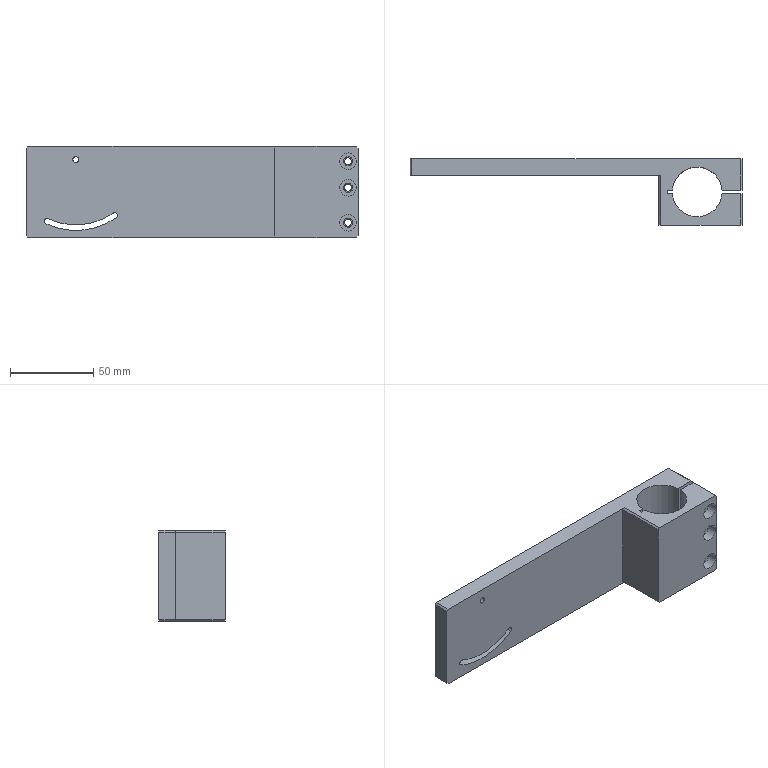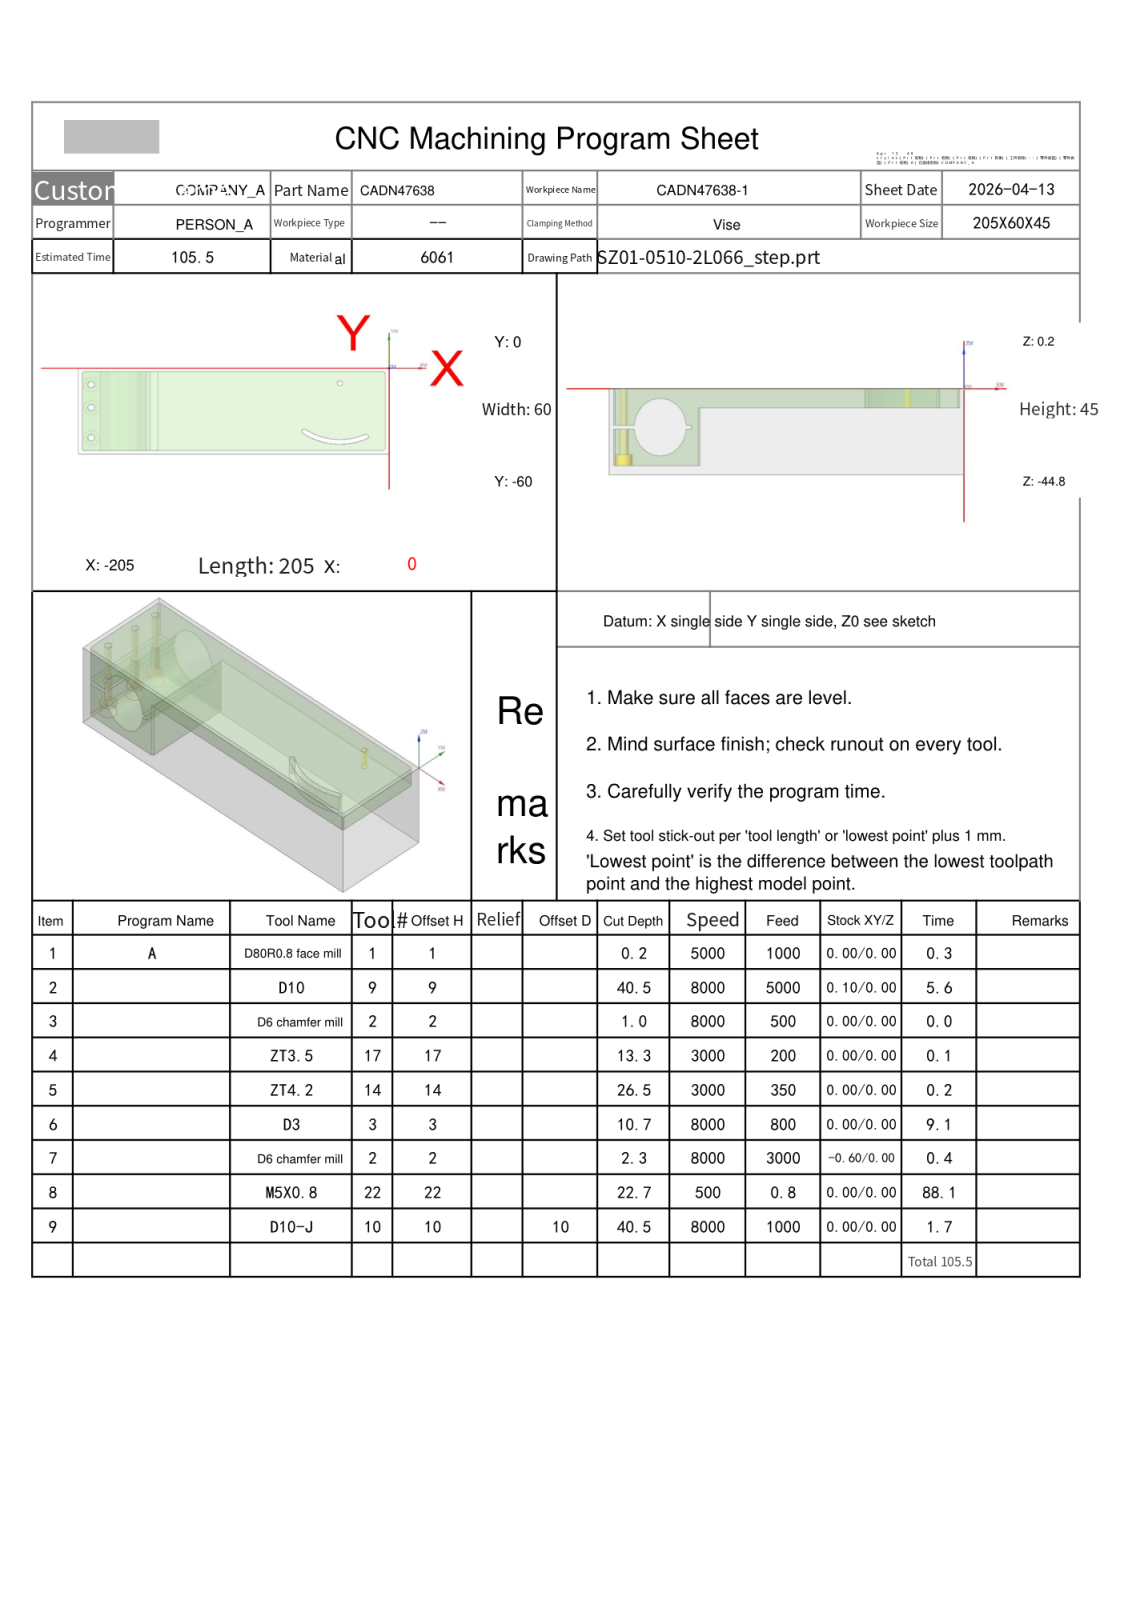NC program | NX | posted by the shop | part box 200 x 40 x 55 mm
Lines 1 to 1033 of 2500:
%
O0001
(Machine time: 191.78 MIN)
(===Total Tool:8===)
(T1=D80R0.8 face mill D=80. R=0.8 D-H01 Z=0.    )
(T9=D10     D=10.  R=0.   D-  H09 Z=-40.3 )
(T2=D6 chamfer mill D=6. R=0. D-H02 Z=-2.05 )
(T17=ZT3.5  D=3.5  DR_a=118 D-  H17 Z=-13.05)
(T14=ZT4.2  D=4.2  DR_a=118 D-  H14 Z=-26.26)
(T3=D3      D=3.   R=0.   D3  H03 Z=-10.5 )
(T22=M5X0.8 D=4.2  DR_a=180 D-  H22 Z=-22.5 )
(T10=D10-J  D=10.  R=0.   D10 H10 Z=-40.3 )
G80 G90 G17 G49 G40
G91 G28 Z0
M01
N1 T01 M06
(D80R0.8 face mill D=80. R=0.8 H=01 ce=0.00 di=0.00)
(MAX_Z=20. MIN_Z=0. Time=0.31M)
G00 G90 G54 X-247.5 Y-30. M03 S5000
G43 H01 Z20.
M08
Z2.
G01 Z0.0 F1000.
X-242.5
X37.5
X42.5
Z2.
G00 Z20.
G91 G28 Z0.0
M05
M09
G91 G28 Z0.0
M01
N2 T09 M06
(D10  D=10. R=0. H=09 ce=0.10 di=0.00)
(MAX_Z=20. MIN_Z=-40.3 Time=5.63M)
G00 G90 G54 X-102.622 Y-62.6 M03 S8000
G43 H09 Z20.
M08
Z.5
G01 X-201.5 Z.353 F5000.
G02 X-201.744 Y-62.594 Z.353 I0.0 J5.1
X-205.106 Y-61.106 Z.347 I.244 J5.094
G01 X-206.106 Y-60.106 Z.345
G02 X-207.6 Y-56.5 Z.339 I3.606 J3.606
G01 Y-3.5 Z.261
G02 X-206.106 Y.106 Z.255 I5.1 J0.0
G01 X-205.106 Y1.106 Z.253
G02 X-201.744 Y2.594 Z.247 I3.606 J-3.606
X-201.5 Y2.6 Z.247 I.244 J-5.094
G01 X-3.5 Z-.047
G02 X.106 Y1.106 Z-.053 I0.0 J-5.1
G01 X1.106 Y.106 Z-.055
G02 X2.6 Y-3.5 Z-.061 I-3.606 J-3.606
G01 Y-56.5 Z-.139
G02 X1.106 Y-60.106 Z-.145 I-5.1 J0.0
G01 X.106 Y-61.106 Z-.147
G02 X-3.5 Y-62.6 Z-.153 I-3.606 J3.606
G01 X-201.5 Z-.447
G02 X-201.744 Y-62.594 Z-.447 I0.0 J5.1
X-205.106 Y-61.106 Z-.453 I.244 J5.094
G01 X-206.106 Y-60.106 Z-.455
G02 X-207.6 Y-56.5 Z-.461 I3.606 J3.606
G01 Y-3.5 Z-.539
G02 X-206.106 Y.106 Z-.545 I5.1 J0.0
G01 X-205.106 Y1.106 Z-.547
G02 X-201.744 Y2.594 Z-.553 I3.606 J-3.606
X-201.5 Y2.6 Z-.553 I.244 J-5.094
G01 X-3.5 Z-.847
G02 X.106 Y1.106 Z-.853 I0.0 J-5.1
G01 X1.106 Y.106 Z-.855
G02 X2.6 Y-3.5 Z-.861 I-3.606 J-3.606
G01 Y-56.5 Z-.939
G02 X1.106 Y-60.106 Z-.945 I-5.1 J0.0
G01 X.106 Y-61.106 Z-.947
G02 X-3.5 Y-62.6 Z-.953 I-3.606 J3.606
G01 X-201.5 Z-1.247
G02 X-201.744 Y-62.594 Z-1.247 I0.0 J5.1
X-205.106 Y-61.106 Z-1.253 I.244 J5.094
G01 X-206.106 Y-60.106 Z-1.255
G02 X-207.6 Y-56.5 Z-1.261 I3.606 J3.606
G01 Y-3.5 Z-1.339
G02 X-206.106 Y.106 Z-1.345 I5.1 J0.0
G01 X-205.106 Y1.106 Z-1.347
G02 X-201.744 Y2.594 Z-1.353 I3.606 J-3.606
X-201.5 Y2.6 Z-1.353 I.244 J-5.094
G01 X-3.5 Z-1.647
G02 X.106 Y1.106 Z-1.653 I0.0 J-5.1
G01 X1.106 Y.106 Z-1.655
G02 X2.6 Y-3.5 Z-1.661 I-3.606 J-3.606
G01 Y-56.5 Z-1.739
G02 X1.106 Y-60.106 Z-1.745 I-5.1 J0.0
G01 X.106 Y-61.106 Z-1.747
G02 X-3.5 Y-62.6 Z-1.753 I-3.606 J3.606
G01 X-201.5 Z-2.047
G02 X-201.744 Y-62.594 Z-2.047 I0.0 J5.1
X-205.106 Y-61.106 Z-2.053 I.244 J5.094
G01 X-206.106 Y-60.106 Z-2.055
G02 X-207.6 Y-56.5 Z-2.061 I3.606 J3.606
G01 Y-3.5 Z-2.139
G02 X-206.106 Y.106 Z-2.145 I5.1 J0.0
G01 X-205.106 Y1.106 Z-2.147
G02 X-201.744 Y2.594 Z-2.153 I3.606 J-3.606
X-201.5 Y2.6 Z-2.153 I.244 J-5.094
G01 X-3.5 Z-2.447
G02 X.106 Y1.106 Z-2.453 I0.0 J-5.1
G01 X1.106 Y.106 Z-2.455
G02 X2.6 Y-3.5 Z-2.461 I-3.606 J-3.606
G01 Y-56.5 Z-2.539
G02 X1.106 Y-60.106 Z-2.545 I-5.1 J0.0
G01 X.106 Y-61.106 Z-2.547
G02 X-3.5 Y-62.6 Z-2.553 I-3.606 J3.606
G01 X-201.5 Z-2.847
G02 X-201.744 Y-62.594 Z-2.847 I0.0 J5.1
X-205.106 Y-61.106 Z-2.853 I.244 J5.094
G01 X-206.106 Y-60.106 Z-2.855
G02 X-207.6 Y-56.5 Z-2.861 I3.606 J3.606
G01 Y-3.5 Z-2.939
G02 X-206.106 Y.106 Z-2.945 I5.1 J0.0
G01 X-205.106 Y1.106 Z-2.947
G02 X-201.744 Y2.594 Z-2.953 I3.606 J-3.606
X-201.5 Y2.6 Z-2.953 I.244 J-5.094
G01 X-3.5 Z-3.247
G02 X.106 Y1.106 Z-3.253 I0.0 J-5.1
G01 X1.106 Y.106 Z-3.255
G02 X2.6 Y-3.5 Z-3.261 I-3.606 J-3.606
G01 Y-56.5 Z-3.339
G02 X1.106 Y-60.106 Z-3.345 I-5.1 J0.0
G01 X.106 Y-61.106 Z-3.347
G02 X-3.5 Y-62.6 Z-3.353 I-3.606 J3.606
G01 X-201.5 Z-3.647
G02 X-201.744 Y-62.594 Z-3.647 I0.0 J5.1
X-205.106 Y-61.106 Z-3.653 I.244 J5.094
G01 X-206.106 Y-60.106 Z-3.655
G02 X-207.6 Y-56.5 Z-3.661 I3.606 J3.606
G01 Y-3.5 Z-3.739
G02 X-206.106 Y.106 Z-3.745 I5.1 J0.0
G01 X-205.106 Y1.106 Z-3.747
G02 X-201.744 Y2.594 Z-3.753 I3.606 J-3.606
X-201.5 Y2.6 Z-3.753 I.244 J-5.094
G01 X-3.5 Z-4.047
G02 X.106 Y1.106 Z-4.053 I0.0 J-5.1
G01 X1.106 Y.106 Z-4.055
G02 X2.6 Y-3.5 Z-4.061 I-3.606 J-3.606
G01 Y-56.5 Z-4.139
G02 X1.106 Y-60.106 Z-4.145 I-5.1 J0.0
G01 X.106 Y-61.106 Z-4.147
G02 X-3.5 Y-62.6 Z-4.153 I-3.606 J3.606
G01 X-201.5 Z-4.447
G02 X-201.744 Y-62.594 Z-4.447 I0.0 J5.1
X-205.106 Y-61.106 Z-4.453 I.244 J5.094
G01 X-206.106 Y-60.106 Z-4.455
G02 X-207.6 Y-56.5 Z-4.461 I3.606 J3.606
G01 Y-3.5 Z-4.539
G02 X-206.106 Y.106 Z-4.545 I5.1 J0.0
G01 X-205.106 Y1.106 Z-4.547
G02 X-201.744 Y2.594 Z-4.553 I3.606 J-3.606
X-201.5 Y2.6 Z-4.553 I.244 J-5.094
G01 X-3.5 Z-4.847
G02 X.106 Y1.106 Z-4.853 I0.0 J-5.1
G01 X1.106 Y.106 Z-4.855
G02 X2.6 Y-3.5 Z-4.861 I-3.606 J-3.606
G01 Y-56.5 Z-4.939
G02 X1.106 Y-60.106 Z-4.945 I-5.1 J0.0
G01 X.106 Y-61.106 Z-4.947
G02 X-3.5 Y-62.6 Z-4.953 I-3.606 J3.606
G01 X-201.5 Z-5.247
G02 X-201.744 Y-62.594 Z-5.247 I0.0 J5.1
X-205.106 Y-61.106 Z-5.253 I.244 J5.094
G01 X-206.106 Y-60.106 Z-5.255
G02 X-207.6 Y-56.5 Z-5.261 I3.606 J3.606
G01 Y-3.5 Z-5.339
G02 X-206.106 Y.106 Z-5.345 I5.1 J0.0
G01 X-205.106 Y1.106 Z-5.347
G02 X-201.744 Y2.594 Z-5.353 I3.606 J-3.606
X-201.5 Y2.6 Z-5.353 I.244 J-5.094
G01 X-3.5 Z-5.647
G02 X.106 Y1.106 Z-5.653 I0.0 J-5.1
G01 X1.106 Y.106 Z-5.655
G02 X2.6 Y-3.5 Z-5.661 I-3.606 J-3.606
G01 Y-56.5 Z-5.739
G02 X1.106 Y-60.106 Z-5.745 I-5.1 J0.0
G01 X.106 Y-61.106 Z-5.747
G02 X-3.5 Y-62.6 Z-5.753 I-3.606 J3.606
G01 X-201.5 Z-6.047
G02 X-201.744 Y-62.594 Z-6.047 I0.0 J5.1
X-205.106 Y-61.106 Z-6.053 I.244 J5.094
G01 X-206.106 Y-60.106 Z-6.055
G02 X-207.6 Y-56.5 Z-6.061 I3.606 J3.606
G01 Y-3.5 Z-6.139
G02 X-206.106 Y.106 Z-6.145 I5.1 J0.0
G01 X-205.106 Y1.106 Z-6.147
G02 X-201.744 Y2.594 Z-6.153 I3.606 J-3.606
X-201.5 Y2.6 Z-6.153 I.244 J-5.094
G01 X-3.5 Z-6.447
G02 X.106 Y1.106 Z-6.453 I0.0 J-5.1
G01 X1.106 Y.106 Z-6.455
G02 X2.6 Y-3.5 Z-6.461 I-3.606 J-3.606
G01 Y-56.5 Z-6.539
G02 X1.106 Y-60.106 Z-6.545 I-5.1 J0.0
G01 X.106 Y-61.106 Z-6.547
G02 X-3.5 Y-62.6 Z-6.553 I-3.606 J3.606
G01 X-201.5 Z-6.847
G02 X-201.744 Y-62.594 Z-6.847 I0.0 J5.1
X-205.106 Y-61.106 Z-6.853 I.244 J5.094
G01 X-206.106 Y-60.106 Z-6.855
G02 X-207.6 Y-56.5 Z-6.861 I3.606 J3.606
G01 Y-3.5 Z-6.939
G02 X-206.106 Y.106 Z-6.945 I5.1 J0.0
G01 X-205.106 Y1.106 Z-6.947
G02 X-201.744 Y2.594 Z-6.953 I3.606 J-3.606
X-201.5 Y2.6 Z-6.953 I.244 J-5.094
G01 X-3.5 Z-7.247
G02 X.106 Y1.106 Z-7.253 I0.0 J-5.1
G01 X1.106 Y.106 Z-7.255
G02 X2.6 Y-3.5 Z-7.261 I-3.606 J-3.606
G01 Y-56.5 Z-7.339
G02 X1.106 Y-60.106 Z-7.345 I-5.1 J0.0
G01 X.106 Y-61.106 Z-7.347
G02 X-3.5 Y-62.6 Z-7.353 I-3.606 J3.606
G01 X-201.5 Z-7.647
G02 X-201.744 Y-62.594 Z-7.647 I0.0 J5.1
X-205.106 Y-61.106 Z-7.653 I.244 J5.094
G01 X-206.106 Y-60.106 Z-7.655
G02 X-207.6 Y-56.5 Z-7.661 I3.606 J3.606
G01 Y-3.5 Z-7.739
G02 X-206.106 Y.106 Z-7.745 I5.1 J0.0
G01 X-205.106 Y1.106 Z-7.747
G02 X-201.744 Y2.594 Z-7.753 I3.606 J-3.606
X-201.5 Y2.6 Z-7.753 I.244 J-5.094
G01 X-3.5 Z-8.047
G02 X.106 Y1.106 Z-8.053 I0.0 J-5.1
G01 X1.106 Y.106 Z-8.055
G02 X2.6 Y-3.5 Z-8.061 I-3.606 J-3.606
G01 Y-56.5 Z-8.139
G02 X1.106 Y-60.106 Z-8.145 I-5.1 J0.0
G01 X.106 Y-61.106 Z-8.147
G02 X-3.5 Y-62.6 Z-8.153 I-3.606 J3.606
G01 X-201.5 Z-8.447
G02 X-201.744 Y-62.594 Z-8.447 I0.0 J5.1
X-205.106 Y-61.106 Z-8.453 I.244 J5.094
G01 X-206.106 Y-60.106 Z-8.455
G02 X-207.6 Y-56.5 Z-8.461 I3.606 J3.606
G01 Y-3.5 Z-8.539
G02 X-206.106 Y.106 Z-8.545 I5.1 J0.0
G01 X-205.106 Y1.106 Z-8.547
G02 X-201.744 Y2.594 Z-8.553 I3.606 J-3.606
X-201.5 Y2.6 Z-8.553 I.244 J-5.094
G01 X-3.5 Z-8.847
G02 X.106 Y1.106 Z-8.853 I0.0 J-5.1
G01 X1.106 Y.106 Z-8.855
G02 X2.6 Y-3.5 Z-8.861 I-3.606 J-3.606
G01 Y-56.5 Z-8.939
G02 X1.106 Y-60.106 Z-8.945 I-5.1 J0.0
G01 X.106 Y-61.106 Z-8.947
G02 X-3.5 Y-62.6 Z-8.953 I-3.606 J3.606
G01 X-201.5 Z-9.247
G02 X-201.744 Y-62.594 Z-9.247 I0.0 J5.1
X-205.106 Y-61.106 Z-9.253 I.244 J5.094
G01 X-206.106 Y-60.106 Z-9.255
G02 X-207.6 Y-56.5 Z-9.261 I3.606 J3.606
G01 Y-3.5 Z-9.339
G02 X-206.106 Y.106 Z-9.345 I5.1 J0.0
G01 X-205.106 Y1.106 Z-9.347
G02 X-201.744 Y2.594 Z-9.353 I3.606 J-3.606
X-201.5 Y2.6 Z-9.353 I.244 J-5.094
G01 X-3.5 Z-9.647
G02 X.106 Y1.106 Z-9.653 I0.0 J-5.1
G01 X1.106 Y.106 Z-9.655
G02 X2.6 Y-3.5 Z-9.661 I-3.606 J-3.606
G01 Y-56.5 Z-9.739
G02 X1.106 Y-60.106 Z-9.745 I-5.1 J0.0
G01 X.106 Y-61.106 Z-9.747
G02 X-3.5 Y-62.6 Z-9.753 I-3.606 J3.606
G01 X-201.5 Z-10.047
G02 X-201.744 Y-62.594 Z-10.047 I0.0 J5.1
X-205.106 Y-61.106 Z-10.053 I.244 J5.094
G01 X-206.106 Y-60.106 Z-10.055
G02 X-207.6 Y-56.5 Z-10.061 I3.606 J3.606
G01 Y-3.5 Z-10.139
G02 X-206.106 Y.106 Z-10.145 I5.1 J0.0
G01 X-205.106 Y1.106 Z-10.147
G02 X-201.744 Y2.594 Z-10.153 I3.606 J-3.606
X-201.5 Y2.6 Z-10.153 I.244 J-5.094
G01 X-3.5 Z-10.447
G02 X.106 Y1.106 Z-10.453 I0.0 J-5.1
G01 X1.106 Y.106 Z-10.455
G02 X2.6 Y-3.5 Z-10.461 I-3.606 J-3.606
G01 Y-56.5 Z-10.539
G02 X1.106 Y-60.106 Z-10.545 I-5.1 J0.0
G01 X.106 Y-61.106 Z-10.547
G02 X-3.5 Y-62.6 Z-10.553 I-3.606 J3.606
G01 X-201.5 Z-10.847
G02 X-201.744 Y-62.594 Z-10.847 I0.0 J5.1
X-205.106 Y-61.106 Z-10.853 I.244 J5.094
G01 X-206.106 Y-60.106 Z-10.855
G02 X-207.6 Y-56.5 Z-10.861 I3.606 J3.606
G01 Y-3.5 Z-10.939
G02 X-206.106 Y.106 Z-10.945 I5.1 J0.0
G01 X-205.106 Y1.106 Z-10.947
G02 X-201.744 Y2.594 Z-10.953 I3.606 J-3.606
X-201.5 Y2.6 Z-10.953 I.244 J-5.094
G01 X-3.5 Z-11.247
G02 X.106 Y1.106 Z-11.253 I0.0 J-5.1
G01 X1.106 Y.106 Z-11.255
G02 X2.6 Y-3.5 Z-11.261 I-3.606 J-3.606
G01 Y-56.5 Z-11.339
G02 X1.106 Y-60.106 Z-11.345 I-5.1 J0.0
G01 X.106 Y-61.106 Z-11.347
G02 X-3.5 Y-62.6 Z-11.353 I-3.606 J3.606
G01 X-201.5 Z-11.647
G02 X-201.744 Y-62.594 Z-11.647 I0.0 J5.1
X-205.106 Y-61.106 Z-11.653 I.244 J5.094
G01 X-206.106 Y-60.106 Z-11.655
G02 X-207.6 Y-56.5 Z-11.661 I3.606 J3.606
G01 Y-3.5 Z-11.739
G02 X-206.106 Y.106 Z-11.745 I5.1 J0.0
G01 X-205.106 Y1.106 Z-11.747
G02 X-201.744 Y2.594 Z-11.753 I3.606 J-3.606
X-201.5 Y2.6 Z-11.753 I.244 J-5.094
G01 X-3.5 Z-12.047
G02 X.106 Y1.106 Z-12.053 I0.0 J-5.1
G01 X1.106 Y.106 Z-12.055
G02 X2.6 Y-3.5 Z-12.061 I-3.606 J-3.606
G01 Y-56.5 Z-12.139
G02 X1.106 Y-60.106 Z-12.145 I-5.1 J0.0
G01 X.106 Y-61.106 Z-12.147
G02 X-3.5 Y-62.6 Z-12.153 I-3.606 J3.606
G01 X-201.5 Z-12.447
G02 X-201.744 Y-62.594 Z-12.447 I0.0 J5.1
X-205.106 Y-61.106 Z-12.453 I.244 J5.094
G01 X-206.106 Y-60.106 Z-12.455
G02 X-207.6 Y-56.5 Z-12.461 I3.606 J3.606
G01 Y-3.5 Z-12.539
G02 X-206.106 Y.106 Z-12.545 I5.1 J0.0
G01 X-205.106 Y1.106 Z-12.547
G02 X-201.744 Y2.594 Z-12.553 I3.606 J-3.606
X-201.5 Y2.6 Z-12.553 I.244 J-5.094
G01 X-3.5 Z-12.847
G02 X.106 Y1.106 Z-12.853 I0.0 J-5.1
G01 X1.106 Y.106 Z-12.855
G02 X2.6 Y-3.5 Z-12.861 I-3.606 J-3.606
G01 Y-56.5 Z-12.939
G02 X1.106 Y-60.106 Z-12.945 I-5.1 J0.0
G01 X.106 Y-61.106 Z-12.947
G02 X-3.5 Y-62.6 Z-12.953 I-3.606 J3.606
G01 X-201.5 Z-13.247
G02 X-201.744 Y-62.594 Z-13.247 I0.0 J5.1
X-205.106 Y-61.106 Z-13.253 I.244 J5.094
G01 X-206.106 Y-60.106 Z-13.255
G02 X-207.6 Y-56.5 Z-13.261 I3.606 J3.606
G01 Y-3.5 Z-13.339
G02 X-206.106 Y.106 Z-13.345 I5.1 J0.0
G01 X-205.106 Y1.106 Z-13.347
G02 X-201.744 Y2.594 Z-13.353 I3.606 J-3.606
X-201.5 Y2.6 Z-13.353 I.244 J-5.094
G01 X-3.5 Z-13.647
G02 X.106 Y1.106 Z-13.653 I0.0 J-5.1
G01 X1.106 Y.106 Z-13.655
G02 X2.6 Y-3.5 Z-13.661 I-3.606 J-3.606
G01 Y-56.5 Z-13.739
G02 X1.106 Y-60.106 Z-13.745 I-5.1 J0.0
G01 X.106 Y-61.106 Z-13.747
G02 X-3.5 Y-62.6 Z-13.753 I-3.606 J3.606
G01 X-201.5 Z-14.047
G02 X-201.744 Y-62.594 Z-14.047 I0.0 J5.1
X-205.106 Y-61.106 Z-14.053 I.244 J5.094
G01 X-206.106 Y-60.106 Z-14.055
G02 X-207.6 Y-56.5 Z-14.061 I3.606 J3.606
G01 Y-3.5 Z-14.139
G02 X-206.106 Y.106 Z-14.145 I5.1 J0.0
G01 X-205.106 Y1.106 Z-14.147
G02 X-201.744 Y2.594 Z-14.153 I3.606 J-3.606
X-201.5 Y2.6 Z-14.153 I.244 J-5.094
G01 X-3.5 Z-14.447
G02 X.106 Y1.106 Z-14.453 I0.0 J-5.1
G01 X1.106 Y.106 Z-14.455
G02 X2.6 Y-3.5 Z-14.461 I-3.606 J-3.606
G01 Y-56.5 Z-14.539
G02 X1.106 Y-60.106 Z-14.545 I-5.1 J0.0
G01 X.106 Y-61.106 Z-14.547
G02 X-3.5 Y-62.6 Z-14.553 I-3.606 J3.606
G01 X-201.5 Z-14.847
G02 X-201.744 Y-62.594 Z-14.847 I0.0 J5.1
X-205.106 Y-61.106 Z-14.853 I.244 J5.094
G01 X-206.106 Y-60.106 Z-14.855
G02 X-207.6 Y-56.5 Z-14.861 I3.606 J3.606
G01 Y-3.5 Z-14.939
G02 X-206.106 Y.106 Z-14.945 I5.1 J0.0
G01 X-205.106 Y1.106 Z-14.947
G02 X-201.744 Y2.594 Z-14.953 I3.606 J-3.606
X-201.5 Y2.6 Z-14.953 I.244 J-5.094
G01 X-3.5 Z-15.247
G02 X.106 Y1.106 Z-15.253 I0.0 J-5.1
G01 X1.106 Y.106 Z-15.255
G02 X2.6 Y-3.5 Z-15.261 I-3.606 J-3.606
G01 Y-56.5 Z-15.339
G02 X1.106 Y-60.106 Z-15.345 I-5.1 J0.0
G01 X.106 Y-61.106 Z-15.347
G02 X-3.5 Y-62.6 Z-15.353 I-3.606 J3.606
G01 X-201.5 Z-15.647
G02 X-201.744 Y-62.594 Z-15.647 I0.0 J5.1
X-205.106 Y-61.106 Z-15.653 I.244 J5.094
G01 X-206.106 Y-60.106 Z-15.655
G02 X-207.6 Y-56.5 Z-15.661 I3.606 J3.606
G01 Y-3.5 Z-15.739
G02 X-206.106 Y.106 Z-15.745 I5.1 J0.0
G01 X-205.106 Y1.106 Z-15.747
G02 X-201.744 Y2.594 Z-15.753 I3.606 J-3.606
X-201.5 Y2.6 Z-15.753 I.244 J-5.094
G01 X-3.5 Z-16.047
G02 X.106 Y1.106 Z-16.053 I0.0 J-5.1
G01 X1.106 Y.106 Z-16.055
G02 X2.6 Y-3.5 Z-16.061 I-3.606 J-3.606
G01 Y-56.5 Z-16.139
G02 X1.106 Y-60.106 Z-16.145 I-5.1 J0.0
G01 X.106 Y-61.106 Z-16.147
G02 X-3.5 Y-62.6 Z-16.153 I-3.606 J3.606
G01 X-201.5 Z-16.447
G02 X-201.744 Y-62.594 Z-16.447 I0.0 J5.1
X-205.106 Y-61.106 Z-16.453 I.244 J5.094
G01 X-206.106 Y-60.106 Z-16.455
G02 X-207.6 Y-56.5 Z-16.461 I3.606 J3.606
G01 Y-3.5 Z-16.539
G02 X-206.106 Y.106 Z-16.545 I5.1 J0.0
G01 X-205.106 Y1.106 Z-16.547
G02 X-201.744 Y2.594 Z-16.553 I3.606 J-3.606
X-201.5 Y2.6 Z-16.553 I.244 J-5.094
G01 X-3.5 Z-16.847
G02 X.106 Y1.106 Z-16.853 I0.0 J-5.1
G01 X1.106 Y.106 Z-16.855
G02 X2.6 Y-3.5 Z-16.861 I-3.606 J-3.606
G01 Y-56.5 Z-16.939
G02 X1.106 Y-60.106 Z-16.945 I-5.1 J0.0
G01 X.106 Y-61.106 Z-16.947
G02 X-3.5 Y-62.6 Z-16.953 I-3.606 J3.606
G01 X-201.5 Z-17.247
G02 X-201.744 Y-62.594 Z-17.247 I0.0 J5.1
X-205.106 Y-61.106 Z-17.253 I.244 J5.094
G01 X-206.106 Y-60.106 Z-17.255
G02 X-207.6 Y-56.5 Z-17.261 I3.606 J3.606
G01 Y-3.5 Z-17.339
G02 X-206.106 Y.106 Z-17.345 I5.1 J0.0
G01 X-205.106 Y1.106 Z-17.347
G02 X-201.744 Y2.594 Z-17.353 I3.606 J-3.606
X-201.5 Y2.6 Z-17.353 I.244 J-5.094
G01 X-3.5 Z-17.647
G02 X.106 Y1.106 Z-17.653 I0.0 J-5.1
G01 X1.106 Y.106 Z-17.655
G02 X2.6 Y-3.5 Z-17.661 I-3.606 J-3.606
G01 Y-56.5 Z-17.739
G02 X1.106 Y-60.106 Z-17.745 I-5.1 J0.0
G01 X.106 Y-61.106 Z-17.747
G02 X-3.5 Y-62.6 Z-17.753 I-3.606 J3.606
G01 X-201.5 Z-18.047
G02 X-201.744 Y-62.594 Z-18.047 I0.0 J5.1
X-205.106 Y-61.106 Z-18.053 I.244 J5.094
G01 X-206.106 Y-60.106 Z-18.055
G02 X-207.6 Y-56.5 Z-18.061 I3.606 J3.606
G01 Y-3.5 Z-18.139
G02 X-206.106 Y.106 Z-18.145 I5.1 J0.0
G01 X-205.106 Y1.106 Z-18.147
G02 X-201.744 Y2.594 Z-18.153 I3.606 J-3.606
X-201.5 Y2.6 Z-18.153 I.244 J-5.094
G01 X-3.5 Z-18.447
G02 X.106 Y1.106 Z-18.453 I0.0 J-5.1
G01 X1.106 Y.106 Z-18.455
G02 X2.6 Y-3.5 Z-18.461 I-3.606 J-3.606
G01 Y-56.5 Z-18.539
G02 X1.106 Y-60.106 Z-18.545 I-5.1 J0.0
G01 X.106 Y-61.106 Z-18.547
G02 X-3.5 Y-62.6 Z-18.553 I-3.606 J3.606
G01 X-201.5 Z-18.847
G02 X-201.744 Y-62.594 Z-18.847 I0.0 J5.1
X-205.106 Y-61.106 Z-18.853 I.244 J5.094
G01 X-206.106 Y-60.106 Z-18.855
G02 X-207.6 Y-56.5 Z-18.861 I3.606 J3.606
G01 Y-3.5 Z-18.939
G02 X-206.106 Y.106 Z-18.945 I5.1 J0.0
G01 X-205.106 Y1.106 Z-18.947
G02 X-201.744 Y2.594 Z-18.953 I3.606 J-3.606
X-201.5 Y2.6 Z-18.953 I.244 J-5.094
G01 X-3.5 Z-19.247
G02 X.106 Y1.106 Z-19.253 I0.0 J-5.1
G01 X1.106 Y.106 Z-19.255
G02 X2.6 Y-3.5 Z-19.261 I-3.606 J-3.606
G01 Y-56.5 Z-19.339
G02 X1.106 Y-60.106 Z-19.345 I-5.1 J0.0
G01 X.106 Y-61.106 Z-19.347
G02 X-3.5 Y-62.6 Z-19.353 I-3.606 J3.606
G01 X-201.5 Z-19.647
G02 X-201.744 Y-62.594 Z-19.647 I0.0 J5.1
X-205.106 Y-61.106 Z-19.653 I.244 J5.094
G01 X-206.106 Y-60.106 Z-19.655
G02 X-207.6 Y-56.5 Z-19.661 I3.606 J3.606
G01 Y-3.5 Z-19.739
G02 X-206.106 Y.106 Z-19.745 I5.1 J0.0
G01 X-205.106 Y1.106 Z-19.747
G02 X-201.744 Y2.594 Z-19.753 I3.606 J-3.606
X-201.5 Y2.6 Z-19.753 I.244 J-5.094
G01 X-3.5 Z-20.047
G02 X.106 Y1.106 Z-20.053 I0.0 J-5.1
G01 X1.106 Y.106 Z-20.055
G02 X2.6 Y-3.5 Z-20.061 I-3.606 J-3.606
G01 Y-56.5 Z-20.139
G02 X1.106 Y-60.106 Z-20.145 I-5.1 J0.0
G01 X.106 Y-61.106 Z-20.147
G02 X-3.5 Y-62.6 Z-20.153 I-3.606 J3.606
G01 X-201.5 Z-20.447
G02 X-201.744 Y-62.594 Z-20.447 I0.0 J5.1
X-205.106 Y-61.106 Z-20.453 I.244 J5.094
G01 X-206.106 Y-60.106 Z-20.455
G02 X-207.6 Y-56.5 Z-20.461 I3.606 J3.606
G01 Y-3.5 Z-20.539
G02 X-206.106 Y.106 Z-20.545 I5.1 J0.0
G01 X-205.106 Y1.106 Z-20.547
G02 X-201.744 Y2.594 Z-20.553 I3.606 J-3.606
X-201.5 Y2.6 Z-20.553 I.244 J-5.094
G01 X-3.5 Z-20.847
G02 X.106 Y1.106 Z-20.853 I0.0 J-5.1
G01 X1.106 Y.106 Z-20.855
G02 X2.6 Y-3.5 Z-20.861 I-3.606 J-3.606
G01 Y-56.5 Z-20.939
G02 X1.106 Y-60.106 Z-20.945 I-5.1 J0.0
G01 X.106 Y-61.106 Z-20.947
G02 X-3.5 Y-62.6 Z-20.953 I-3.606 J3.606
G01 X-201.5 Z-21.247
G02 X-201.744 Y-62.594 Z-21.247 I0.0 J5.1
X-205.106 Y-61.106 Z-21.253 I.244 J5.094
G01 X-206.106 Y-60.106 Z-21.255
G02 X-207.6 Y-56.5 Z-21.261 I3.606 J3.606
G01 Y-3.5 Z-21.339
G02 X-206.106 Y.106 Z-21.345 I5.1 J0.0
G01 X-205.106 Y1.106 Z-21.347
G02 X-201.744 Y2.594 Z-21.353 I3.606 J-3.606
X-201.5 Y2.6 Z-21.353 I.244 J-5.094
G01 X-3.5 Z-21.647
G02 X.106 Y1.106 Z-21.653 I0.0 J-5.1
G01 X1.106 Y.106 Z-21.655
G02 X2.6 Y-3.5 Z-21.661 I-3.606 J-3.606
G01 Y-56.5 Z-21.739
G02 X1.106 Y-60.106 Z-21.745 I-5.1 J0.0
G01 X.106 Y-61.106 Z-21.747
G02 X-3.5 Y-62.6 Z-21.753 I-3.606 J3.606
G01 X-201.5 Z-22.047
G02 X-201.744 Y-62.594 Z-22.047 I0.0 J5.1
X-205.106 Y-61.106 Z-22.053 I.244 J5.094
G01 X-206.106 Y-60.106 Z-22.055
G02 X-207.6 Y-56.5 Z-22.061 I3.606 J3.606
G01 Y-3.5 Z-22.139
G02 X-206.106 Y.106 Z-22.145 I5.1 J0.0
G01 X-205.106 Y1.106 Z-22.147
G02 X-201.744 Y2.594 Z-22.153 I3.606 J-3.606
X-201.5 Y2.6 Z-22.153 I.244 J-5.094
G01 X-3.5 Z-22.447
G02 X.106 Y1.106 Z-22.453 I0.0 J-5.1
G01 X1.106 Y.106 Z-22.455
G02 X2.6 Y-3.5 Z-22.461 I-3.606 J-3.606
G01 Y-56.5 Z-22.539
G02 X1.106 Y-60.106 Z-22.545 I-5.1 J0.0
G01 X.106 Y-61.106 Z-22.547
G02 X-3.5 Y-62.6 Z-22.553 I-3.606 J3.606
G01 X-201.5 Z-22.847
G02 X-201.744 Y-62.594 Z-22.847 I0.0 J5.1
X-205.106 Y-61.106 Z-22.853 I.244 J5.094
G01 X-206.106 Y-60.106 Z-22.855
G02 X-207.6 Y-56.5 Z-22.861 I3.606 J3.606
G01 Y-3.5 Z-22.939
G02 X-206.106 Y.106 Z-22.945 I5.1 J0.0
G01 X-205.106 Y1.106 Z-22.947
G02 X-201.744 Y2.594 Z-22.953 I3.606 J-3.606
X-201.5 Y2.6 Z-22.953 I.244 J-5.094
G01 X-3.5 Z-23.247
G02 X.106 Y1.106 Z-23.253 I0.0 J-5.1
G01 X1.106 Y.106 Z-23.255
G02 X2.6 Y-3.5 Z-23.261 I-3.606 J-3.606
G01 Y-56.5 Z-23.339
G02 X1.106 Y-60.106 Z-23.345 I-5.1 J0.0
G01 X.106 Y-61.106 Z-23.347
G02 X-3.5 Y-62.6 Z-23.353 I-3.606 J3.606
G01 X-201.5 Z-23.647
G02 X-201.744 Y-62.594 Z-23.647 I0.0 J5.1
X-205.106 Y-61.106 Z-23.653 I.244 J5.094
G01 X-206.106 Y-60.106 Z-23.655
G02 X-207.6 Y-56.5 Z-23.661 I3.606 J3.606
G01 Y-3.5 Z-23.739
G02 X-206.106 Y.106 Z-23.745 I5.1 J0.0
G01 X-205.106 Y1.106 Z-23.747
G02 X-201.744 Y2.594 Z-23.753 I3.606 J-3.606
X-201.5 Y2.6 Z-23.753 I.244 J-5.094
G01 X-3.5 Z-24.047
G02 X.106 Y1.106 Z-24.053 I0.0 J-5.1
G01 X1.106 Y.106 Z-24.055
G02 X2.6 Y-3.5 Z-24.061 I-3.606 J-3.606
G01 Y-56.5 Z-24.139
G02 X1.106 Y-60.106 Z-24.145 I-5.1 J0.0
G01 X.106 Y-61.106 Z-24.147
G02 X-3.5 Y-62.6 Z-24.153 I-3.606 J3.606
G01 X-201.5 Z-24.447
G02 X-201.744 Y-62.594 Z-24.447 I0.0 J5.1
X-205.106 Y-61.106 Z-24.453 I.244 J5.094
G01 X-206.106 Y-60.106 Z-24.455
G02 X-207.6 Y-56.5 Z-24.461 I3.606 J3.606
G01 Y-3.5 Z-24.539
G02 X-206.106 Y.106 Z-24.545 I5.1 J0.0
G01 X-205.106 Y1.106 Z-24.547
G02 X-201.744 Y2.594 Z-24.553 I3.606 J-3.606
X-201.5 Y2.6 Z-24.553 I.244 J-5.094
G01 X-3.5 Z-24.847
G02 X.106 Y1.106 Z-24.853 I0.0 J-5.1
G01 X1.106 Y.106 Z-24.855
G02 X2.6 Y-3.5 Z-24.861 I-3.606 J-3.606
G01 Y-56.5 Z-24.939
G02 X1.106 Y-60.106 Z-24.945 I-5.1 J0.0
G01 X.106 Y-61.106 Z-24.947
G02 X-3.5 Y-62.6 Z-24.953 I-3.606 J3.606
G01 X-201.5 Z-25.247
G02 X-201.744 Y-62.594 Z-25.247 I0.0 J5.1
X-205.106 Y-61.106 Z-25.253 I.244 J5.094
G01 X-206.106 Y-60.106 Z-25.255
G02 X-207.6 Y-56.5 Z-25.261 I3.606 J3.606
G01 Y-3.5 Z-25.339
G02 X-206.106 Y.106 Z-25.345 I5.1 J0.0
G01 X-205.106 Y1.106 Z-25.347
G02 X-201.744 Y2.594 Z-25.353 I3.606 J-3.606
X-201.5 Y2.6 Z-25.353 I.244 J-5.094
G01 X-3.5 Z-25.647
G02 X.106 Y1.106 Z-25.653 I0.0 J-5.1
G01 X1.106 Y.106 Z-25.655
G02 X2.6 Y-3.5 Z-25.661 I-3.606 J-3.606
G01 Y-56.5 Z-25.739
G02 X1.106 Y-60.106 Z-25.745 I-5.1 J0.0
G01 X.106 Y-61.106 Z-25.747
G02 X-3.5 Y-62.6 Z-25.753 I-3.606 J3.606
G01 X-201.5 Z-26.047
G02 X-201.744 Y-62.594 Z-26.047 I0.0 J5.1
X-205.106 Y-61.106 Z-26.053 I.244 J5.094
G01 X-206.106 Y-60.106 Z-26.055
G02 X-207.6 Y-56.5 Z-26.061 I3.606 J3.606
G01 Y-3.5 Z-26.139
G02 X-206.106 Y.106 Z-26.145 I5.1 J0.0
G01 X-205.106 Y1.106 Z-26.147
G02 X-201.744 Y2.594 Z-26.153 I3.606 J-3.606
X-201.5 Y2.6 Z-26.153 I.244 J-5.094
G01 X-3.5 Z-26.447
G02 X.106 Y1.106 Z-26.453 I0.0 J-5.1
G01 X1.106 Y.106 Z-26.455
G02 X2.6 Y-3.5 Z-26.461 I-3.606 J-3.606
G01 Y-56.5 Z-26.539
G02 X1.106 Y-60.106 Z-26.545 I-5.1 J0.0
G01 X.106 Y-61.106 Z-26.547
G02 X-3.5 Y-62.6 Z-26.553 I-3.606 J3.606
G01 X-201.5 Z-26.847
G02 X-201.744 Y-62.594 Z-26.847 I0.0 J5.1
X-205.106 Y-61.106 Z-26.853 I.244 J5.094
G01 X-206.106 Y-60.106 Z-26.855
G02 X-207.6 Y-56.5 Z-26.861 I3.606 J3.606
G01 Y-3.5 Z-26.939
G02 X-206.106 Y.106 Z-26.945 I5.1 J0.0
G01 X-205.106 Y1.106 Z-26.947
G02 X-201.744 Y2.594 Z-26.953 I3.606 J-3.606
X-201.5 Y2.6 Z-26.953 I.244 J-5.094
G01 X-3.5 Z-27.247
G02 X.106 Y1.106 Z-27.253 I0.0 J-5.1
G01 X1.106 Y.106 Z-27.255
G02 X2.6 Y-3.5 Z-27.261 I-3.606 J-3.606
G01 Y-56.5 Z-27.339
G02 X1.106 Y-60.106 Z-27.345 I-5.1 J0.0
G01 X.106 Y-61.106 Z-27.347
G02 X-3.5 Y-62.6 Z-27.353 I-3.606 J3.606
G01 X-201.5 Z-27.647
G02 X-201.744 Y-62.594 Z-27.647 I0.0 J5.1
X-205.106 Y-61.106 Z-27.653 I.244 J5.094
G01 X-206.106 Y-60.106 Z-27.655
G02 X-207.6 Y-56.5 Z-27.661 I3.606 J3.606
G01 Y-3.5 Z-27.739
G02 X-206.106 Y.106 Z-27.745 I5.1 J0.0
G01 X-205.106 Y1.106 Z-27.747
G02 X-201.744 Y2.594 Z-27.753 I3.606 J-3.606
X-201.5 Y2.6 Z-27.753 I.244 J-5.094
G01 X-3.5 Z-28.047
G02 X.106 Y1.106 Z-28.053 I0.0 J-5.1
G01 X1.106 Y.106 Z-28.055
G02 X2.6 Y-3.5 Z-28.061 I-3.606 J-3.606
G01 Y-56.5 Z-28.139
G02 X1.106 Y-60.106 Z-28.145 I-5.1 J0.0
G01 X.106 Y-61.106 Z-28.147
G02 X-3.5 Y-62.6 Z-28.153 I-3.606 J3.606
G01 X-201.5 Z-28.447
G02 X-201.744 Y-62.594 Z-28.447 I0.0 J5.1
X-205.106 Y-61.106 Z-28.453 I.244 J5.094
G01 X-206.106 Y-60.106 Z-28.455
G02 X-207.6 Y-56.5 Z-28.461 I3.606 J3.606
G01 Y-3.5 Z-28.539
G02 X-206.106 Y.106 Z-28.545 I5.1 J0.0
G01 X-205.106 Y1.106 Z-28.547
G02 X-201.744 Y2.594 Z-28.553 I3.606 J-3.606
X-201.5 Y2.6 Z-28.553 I.244 J-5.094
G01 X-3.5 Z-28.847
G02 X.106 Y1.106 Z-28.853 I0.0 J-5.1
G01 X1.106 Y.106 Z-28.855
G02 X2.6 Y-3.5 Z-28.861 I-3.606 J-3.606
G01 Y-56.5 Z-28.939
G02 X1.106 Y-60.106 Z-28.945 I-5.1 J0.0
G01 X.106 Y-61.106 Z-28.947
G02 X-3.5 Y-62.6 Z-28.953 I-3.606 J3.606
G01 X-201.5 Z-29.247
G02 X-201.744 Y-62.594 Z-29.247 I0.0 J5.1
X-205.106 Y-61.106 Z-29.253 I.244 J5.094
G01 X-206.106 Y-60.106 Z-29.255
G02 X-207.6 Y-56.5 Z-29.261 I3.606 J3.606
G01 Y-3.5 Z-29.339
G02 X-206.106 Y.106 Z-29.345 I5.1 J0.0
G01 X-205.106 Y1.106 Z-29.347
G02 X-201.744 Y2.594 Z-29.353 I3.606 J-3.606
X-201.5 Y2.6 Z-29.353 I.244 J-5.094
G01 X-3.5 Z-29.647
G02 X.106 Y1.106 Z-29.653 I0.0 J-5.1
G01 X1.106 Y.106 Z-29.655
G02 X2.6 Y-3.5 Z-29.661 I-3.606 J-3.606
G01 Y-56.5 Z-29.739
G02 X1.106 Y-60.106 Z-29.745 I-5.1 J0.0
G01 X.106 Y-61.106 Z-29.747
G02 X-3.5 Y-62.6 Z-29.753 I-3.606 J3.606
G01 X-201.5 Z-30.047
G02 X-201.744 Y-62.594 Z-30.047 I0.0 J5.1
X-205.106 Y-61.106 Z-30.053 I.244 J5.094
G01 X-206.106 Y-60.106 Z-30.055
G02 X-207.6 Y-56.5 Z-30.061 I3.606 J3.606
G01 Y-3.5 Z-30.139
G02 X-206.106 Y.106 Z-30.145 I5.1 J0.0
G01 X-205.106 Y1.106 Z-30.147
G02 X-201.744 Y2.594 Z-30.153 I3.606 J-3.606
X-201.5 Y2.6 Z-30.153 I.244 J-5.094
G01 X-3.5 Z-30.447
G02 X.106 Y1.106 Z-30.453 I0.0 J-5.1
G01 X1.106 Y.106 Z-30.455
G02 X2.6 Y-3.5 Z-30.461 I-3.606 J-3.606
G01 Y-56.5 Z-30.539
G02 X1.106 Y-60.106 Z-30.545 I-5.1 J0.0
G01 X.106 Y-61.106 Z-30.547
G02 X-3.5 Y-62.6 Z-30.553 I-3.606 J3.606
G01 X-201.5 Z-30.847
G02 X-201.744 Y-62.594 Z-30.847 I0.0 J5.1
X-205.106 Y-61.106 Z-30.853 I.244 J5.094
G01 X-206.106 Y-60.106 Z-30.855
G02 X-207.6 Y-56.5 Z-30.861 I3.606 J3.606
G01 Y-3.5 Z-30.939
G02 X-206.106 Y.106 Z-30.945 I5.1 J0.0
G01 X-205.106 Y1.106 Z-30.947
G02 X-201.744 Y2.594 Z-30.953 I3.606 J-3.606
X-201.5 Y2.6 Z-30.953 I.244 J-5.094
G01 X-3.5 Z-31.247
G02 X.106 Y1.106 Z-31.253 I0.0 J-5.1
G01 X1.106 Y.106 Z-31.255
G02 X2.6 Y-3.5 Z-31.261 I-3.606 J-3.606
G01 Y-56.5 Z-31.339
G02 X1.106 Y-60.106 Z-31.345 I-5.1 J0.0
G01 X.106 Y-61.106 Z-31.347
G02 X-3.5 Y-62.6 Z-31.353 I-3.606 J3.606
G01 X-201.5 Z-31.647
G02 X-201.744 Y-62.594 Z-31.647 I0.0 J5.1
X-205.106 Y-61.106 Z-31.653 I.244 J5.094
G01 X-206.106 Y-60.106 Z-31.655
G02 X-207.6 Y-56.5 Z-31.661 I3.606 J3.606
G01 Y-3.5 Z-31.739
G02 X-206.106 Y.106 Z-31.745 I5.1 J0.0
G01 X-205.106 Y1.106 Z-31.747
G02 X-201.744 Y2.594 Z-31.753 I3.606 J-3.606
X-201.5 Y2.6 Z-31.753 I.244 J-5.094
G01 X-3.5 Z-32.047
G02 X.106 Y1.106 Z-32.053 I0.0 J-5.1
G01 X1.106 Y.106 Z-32.055
G02 X2.6 Y-3.5 Z-32.061 I-3.606 J-3.606
G01 Y-56.5 Z-32.139
G02 X1.106 Y-60.106 Z-32.145 I-5.1 J0.0
G01 X.106 Y-61.106 Z-32.147
G02 X-3.5 Y-62.6 Z-32.153 I-3.606 J3.606
G01 X-201.5 Z-32.447
G02 X-201.744 Y-62.594 Z-32.447 I0.0 J5.1
X-205.106 Y-61.106 Z-32.453 I.244 J5.094
G01 X-206.106 Y-60.106 Z-32.455
G02 X-207.6 Y-56.5 Z-32.461 I3.606 J3.606
G01 Y-3.5 Z-32.539
G02 X-206.106 Y.106 Z-32.545 I5.1 J0.0
G01 X-205.106 Y1.106 Z-32.547
G02 X-201.744 Y2.594 Z-32.553 I3.606 J-3.606
X-201.5 Y2.6 Z-32.553 I.244 J-5.094
G01 X-3.5 Z-32.847
G02 X.106 Y1.106 Z-32.853 I0.0 J-5.1
G01 X1.106 Y.106 Z-32.855
G02 X2.6 Y-3.5 Z-32.861 I-3.606 J-3.606
G01 Y-56.5 Z-32.939
G02 X1.106 Y-60.106 Z-32.945 I-5.1 J0.0
G01 X.106 Y-61.106 Z-32.947
G02 X-3.5 Y-62.6 Z-32.953 I-3.606 J3.606
G01 X-201.5 Z-33.247
G02 X-201.744 Y-62.594 Z-33.247 I0.0 J5.1
X-205.106 Y-61.106 Z-33.253 I.244 J5.094
G01 X-206.106 Y-60.106 Z-33.255
G02 X-207.6 Y-56.5 Z-33.261 I3.606 J3.606
G01 Y-3.5 Z-33.339
G02 X-206.106 Y.106 Z-33.345 I5.1 J0.0
G01 X-205.106 Y1.106 Z-33.347
G02 X-201.744 Y2.594 Z-33.353 I3.606 J-3.606
X-201.5 Y2.6 Z-33.353 I.244 J-5.094
G01 X-3.5 Z-33.647
G02 X.106 Y1.106 Z-33.653 I0.0 J-5.1
G01 X1.106 Y.106 Z-33.655
G02 X2.6 Y-3.5 Z-33.661 I-3.606 J-3.606
G01 Y-56.5 Z-33.739
G02 X1.106 Y-60.106 Z-33.745 I-5.1 J0.0
G01 X.106 Y-61.106 Z-33.747
G02 X-3.5 Y-62.6 Z-33.753 I-3.606 J3.606
G01 X-201.5 Z-34.047
G02 X-201.744 Y-62.594 Z-34.047 I0.0 J5.1
X-205.106 Y-61.106 Z-34.053 I.244 J5.094
G01 X-206.106 Y-60.106 Z-34.055
G02 X-207.6 Y-56.5 Z-34.061 I3.606 J3.606
G01 Y-3.5 Z-34.139
G02 X-206.106 Y.106 Z-34.145 I5.1 J0.0
G01 X-205.106 Y1.106 Z-34.147
G02 X-201.744 Y2.594 Z-34.153 I3.606 J-3.606
X-201.5 Y2.6 Z-34.153 I.244 J-5.094
G01 X-3.5 Z-34.447
G02 X.106 Y1.106 Z-34.453 I0.0 J-5.1
G01 X1.106 Y.106 Z-34.455
G02 X2.6 Y-3.5 Z-34.461 I-3.606 J-3.606
G01 Y-56.5 Z-34.539
G02 X1.106 Y-60.106 Z-34.545 I-5.1 J0.0
G01 X.106 Y-61.106 Z-34.547
G02 X-3.5 Y-62.6 Z-34.553 I-3.606 J3.606
G01 X-201.5 Z-34.847
G02 X-201.744 Y-62.594 Z-34.847 I0.0 J5.1
X-205.106 Y-61.106 Z-34.853 I.244 J5.094
G01 X-206.106 Y-60.106 Z-34.855
G02 X-207.6 Y-56.5 Z-34.861 I3.606 J3.606
G01 Y-3.5 Z-34.939
G02 X-206.106 Y.106 Z-34.945 I5.1 J0.0
G01 X-205.106 Y1.106 Z-34.947
G02 X-201.744 Y2.594 Z-34.953 I3.606 J-3.606
X-201.5 Y2.6 Z-34.953 I.244 J-5.094
G01 X-3.5 Z-35.247
G02 X.106 Y1.106 Z-35.253 I0.0 J-5.1
G01 X1.106 Y.106 Z-35.255
G02 X2.6 Y-3.5 Z-35.261 I-3.606 J-3.606
G01 Y-56.5 Z-35.339
G02 X1.106 Y-60.106 Z-35.345 I-5.1 J0.0
G01 X.106 Y-61.106 Z-35.347
G02 X-3.5 Y-62.6 Z-35.353 I-3.606 J3.606
G01 X-201.5 Z-35.647
G02 X-201.744 Y-62.594 Z-35.647 I0.0 J5.1
X-205.106 Y-61.106 Z-35.653 I.244 J5.094
G01 X-206.106 Y-60.106 Z-35.655
G02 X-207.6 Y-56.5 Z-35.661 I3.606 J3.606
G01 Y-3.5 Z-35.739
G02 X-206.106 Y.106 Z-35.745 I5.1 J0.0
G01 X-205.106 Y1.106 Z-35.747
G02 X-201.744 Y2.594 Z-35.753 I3.606 J-3.606
X-201.5 Y2.6 Z-35.753 I.244 J-5.094
G01 X-3.5 Z-36.047
G02 X.106 Y1.106 Z-36.053 I0.0 J-5.1
G01 X1.106 Y.106 Z-36.055
G02 X2.6 Y-3.5 Z-36.061 I-3.606 J-3.606
G01 Y-56.5 Z-36.139
G02 X1.106 Y-60.106 Z-36.145 I-5.1 J0.0
G01 X.106 Y-61.106 Z-36.147
G02 X-3.5 Y-62.6 Z-36.153 I-3.606 J3.606
G01 X-201.5 Z-36.447
G02 X-201.744 Y-62.594 Z-36.447 I0.0 J5.1
X-205.106 Y-61.106 Z-36.453 I.244 J5.094
G01 X-206.106 Y-60.106 Z-36.455
G02 X-207.6 Y-56.5 Z-36.461 I3.606 J3.606
G01 Y-3.5 Z-36.539
G02 X-206.106 Y.106 Z-36.545 I5.1 J0.0
G01 X-205.106 Y1.106 Z-36.547
G02 X-201.744 Y2.594 Z-36.553 I3.606 J-3.606
X-201.5 Y2.6 Z-36.553 I.244 J-5.094
G01 X-3.5 Z-36.847
G02 X.106 Y1.106 Z-36.853 I0.0 J-5.1
G01 X1.106 Y.106 Z-36.855
G02 X2.6 Y-3.5 Z-36.861 I-3.606 J-3.606
G01 Y-56.5 Z-36.939
G02 X1.106 Y-60.106 Z-36.945 I-5.1 J0.0
G01 X.106 Y-61.106 Z-36.947
G02 X-3.5 Y-62.6 Z-36.953 I-3.606 J3.606
G01 X-201.5 Z-37.247
G02 X-201.744 Y-62.594 Z-37.247 I0.0 J5.1
X-205.106 Y-61.106 Z-37.253 I.244 J5.094
G01 X-206.106 Y-60.106 Z-37.255
G02 X-207.6 Y-56.5 Z-37.261 I3.606 J3.606
G01 Y-3.5 Z-37.339
G02 X-206.106 Y.106 Z-37.345 I5.1 J0.0
G01 X-205.106 Y1.106 Z-37.347
G02 X-201.744 Y2.594 Z-37.353 I3.606 J-3.606
X-201.5 Y2.6 Z-37.353 I.244 J-5.094
G01 X-3.5 Z-37.647
G02 X.106 Y1.106 Z-37.653 I0.0 J-5.1
G01 X1.106 Y.106 Z-37.655
G02 X2.6 Y-3.5 Z-37.661 I-3.606 J-3.606
G01 Y-56.5 Z-37.739
G02 X1.106 Y-60.106 Z-37.745 I-5.1 J0.0
G01 X.106 Y-61.106 Z-37.747
G02 X-3.5 Y-62.6 Z-37.753 I-3.606 J3.606
G01 X-201.5 Z-38.047
G02 X-201.744 Y-62.594 Z-38.047 I0.0 J5.1
X-205.106 Y-61.106 Z-38.053 I.244 J5.094
G01 X-206.106 Y-60.106 Z-38.055
G02 X-207.6 Y-56.5 Z-38.061 I3.606 J3.606
G01 Y-3.5 Z-38.139
G02 X-206.106 Y.106 Z-38.145 I5.1 J0.0
G01 X-205.106 Y1.106 Z-38.147
G02 X-201.744 Y2.594 Z-38.153 I3.606 J-3.606
X-201.5 Y2.6 Z-38.153 I.244 J-5.094
G01 X-3.5 Z-38.447
G02 X.106 Y1.106 Z-38.453 I0.0 J-5.1
G01 X1.106 Y.106 Z-38.455
G02 X2.6 Y-3.5 Z-38.461 I-3.606 J-3.606
G01 Y-56.5 Z-38.539
G02 X1.106 Y-60.106 Z-38.545 I-5.1 J0.0
G01 X.106 Y-61.106 Z-38.547
G02 X-3.5 Y-62.6 Z-38.553 I-3.606 J3.606
G01 X-201.5 Z-38.847
G02 X-201.744 Y-62.594 Z-38.847 I0.0 J5.1
X-205.106 Y-61.106 Z-38.853 I.244 J5.094
G01 X-206.106 Y-60.106 Z-38.855
G02 X-207.6 Y-56.5 Z-38.861 I3.606 J3.606
G01 Y-3.5 Z-38.939
G02 X-206.106 Y.106 Z-38.945 I5.1 J0.0
G01 X-205.106 Y1.106 Z-38.947
G02 X-201.744 Y2.594 Z-38.953 I3.606 J-3.606
X-201.5 Y2.6 Z-38.953 I.244 J-5.094
G01 X-3.5 Z-39.247
G02 X.106 Y1.106 Z-39.253 I0.0 J-5.1
G01 X1.106 Y.106 Z-39.255
G02 X2.6 Y-3.5 Z-39.261 I-3.606 J-3.606
G01 Y-56.5 Z-39.339
G02 X1.106 Y-60.106 Z-39.345 I-5.1 J0.0
G01 X.106 Y-61.106 Z-39.347
G02 X-3.5 Y-62.6 Z-39.353 I-3.606 J3.606
G01 X-201.5 Z-39.647
G02 X-201.744 Y-62.594 Z-39.647 I0.0 J5.1
X-205.106 Y-61.106 Z-39.653 I.244 J5.094
G01 X-206.106 Y-60.106 Z-39.655
G02 X-207.6 Y-56.5 Z-39.661 I3.606 J3.606
G01 Y-3.5 Z-39.739
G02 X-206.106 Y.106 Z-39.745 I5.1 J0.0
G01 X-205.106 Y1.106 Z-39.747
G02 X-201.744 Y2.594 Z-39.753 I3.606 J-3.606
X-201.5 Y2.6 Z-39.753 I.244 J-5.094
G01 X-3.5 Z-40.047
G02 X.106 Y1.106 Z-40.053 I0.0 J-5.1
G01 X1.106 Y.106 Z-40.055
G02 X2.6 Y-3.5 Z-40.061 I-3.606 J-3.606
G01 Y-56.5 Z-40.139
G02 X1.106 Y-60.106 Z-40.145 I-5.1 J0.0
G01 X.106 Y-61.106 Z-40.147
G02 X-3.5 Y-62.6 Z-40.153 I-3.606 J3.606
G01 X-102.622 Z-40.3
X-201.5
G02 X-205.106 Y-61.106 I0.0 J5.1
G01 X-206.106 Y-60.106
G02 X-207.6 Y-56.5 I3.606 J3.606
G01 Y-3.5
G02 X-206.106 Y.106 I5.1 J0.0
G01 X-205.106 Y1.106
G02 X-201.5 Y2.6 I3.606 J-3.606
G01 X-3.5
G02 X.106 Y1.106 I0.0 J-5.1
G01 X1.106 Y.106
G02 X2.6 Y-3.5 I-3.606 J-3.606
G01 Y-56.5
G02 X1.106 Y-60.106 I-5.1 J0.0
G01 X.106 Y-61.106
G02 X-3.5 Y-62.6 I-3.606 J3.606
G01 X-102.622
X-103.122
Z-39.3
G00 Z20.
G91 G28 Z0.0
M05
M09
G91 G28 Z0.0
M01
N3 T02 M06
(D6 chamfer mill D=6. R=0. H=02 ce=0.00 di=0.00)
(MAX_Z=20. MIN_Z=-0.8 Time=0.04M)
G00 G90 G54 X-32.5 Y-10.5 M03 S8000
G43 H02 Z20.
M08
G98 G81 X-32.5 Y-10.5 Z-.8 R1. F500.
X-196.5 Y-11.5
Y-27.5
Y-48.5
G80
G00 Z20.
G91 G28 Z0.0
M05
M09
G91 G28 Z0.0
M01
N4 T17 M06
(ZT3.5 D=3.5 DR_a=118 H=17)
(MAX_Z=20. MIN_Z=-13.05 Time=0.08M)
G00 G90 G54 X-32.5 Y-10.5 M03 S3000
G43 H17 Z20.
M08
G98 G83 X-32.5 Y-10.5 Z-13.052 R1. F200. Q3.
G80
G00 Z20.
G91 G28 Z0.0
M05
M09
G91 G28 Z0.0
M01
N5 T14 M06
(ZT4.2 D=4.2 DR_a=118 H=14)
(MAX_Z=20. MIN_Z=-26.26 Time=0.25M)
G00 G90 G54 X-196.5 Y-11.5 M03 S3000
G43 H14 Z20.
M08
G98 G83 X-196.5 Y-11.5 Z-26.262 R1. F350. Q3.
Y-27.5
Y-48.5
G80
G00 Z20.
G91 G28 Z0.0
M05
M09
G91 G28 Z0.0
M01